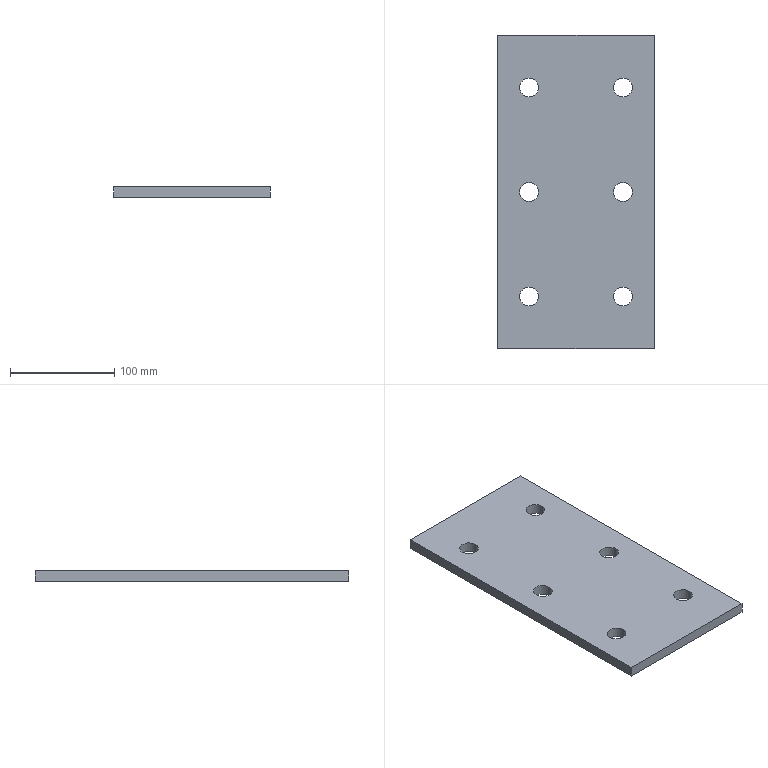Part | SolidWorks | features Extrusion 1 | 1 solid | 18 faces | box 150 x 300 x 10 mm | volume 434732 mm3 | cylinder 12 | plane 6 | commonest cylinder face diameters 18 x12
STEP:
#1=CARTESIAN_POINT('',(36.,100.,10.));
#2=VERTEX_POINT('',#1);
#3=CARTESIAN_POINT('',(54.,100.,10.));
#4=VERTEX_POINT('',#3);
#5=CARTESIAN_POINT('',(45.,100.,10.));
#6=DIRECTION('',(0.,0.,1.));
#7=DIRECTION('',(-1.,0.,0.));
#8=AXIS2_PLACEMENT_3D('',#5,#6,#7);
#9=CIRCLE('',#8,9.);
#10=EDGE_CURVE('',#2,#4,#9,.T.);
#11=ORIENTED_EDGE('',*,*,#10,.T.);
#12=CARTESIAN_POINT('',(54.,100.,0.));
#13=VERTEX_POINT('',#12);
#14=CARTESIAN_POINT('',(54.,100.,10.));
#15=DIRECTION('',(0.,0.,-1.));
#16=VECTOR('',#15,1000.);
#17=LINE('',#14,#16);
#18=EDGE_CURVE('',#4,#13,#17,.T.);
#19=ORIENTED_EDGE('',*,*,#18,.T.);
#20=CARTESIAN_POINT('',(36.,100.,0.));
#21=VERTEX_POINT('',#20);
#22=CARTESIAN_POINT('',(45.,100.,0.));
#23=DIRECTION('',(0.,0.,1.));
#24=DIRECTION('',(-1.,0.,0.));
#25=AXIS2_PLACEMENT_3D('',#22,#23,#24);
#26=CIRCLE('',#25,9.);
#27=EDGE_CURVE('',#21,#13,#26,.T.);
#28=ORIENTED_EDGE('',*,*,#27,.F.);
#29=CARTESIAN_POINT('',(36.,100.,10.));
#30=DIRECTION('',(0.,0.,-1.));
#31=VECTOR('',#30,1000.);
#32=LINE('',#29,#31);
#33=EDGE_CURVE('',#2,#21,#32,.T.);
#34=ORIENTED_EDGE('',*,*,#33,.F.);
#35=EDGE_LOOP('',(#11,#19,#28,#34));
#36=FACE_OUTER_BOUND('',#35,.T.);
#37=CARTESIAN_POINT('',(45.,100.,10.));
#38=DIRECTION('',(0.,0.,-1.));
#39=DIRECTION('',(-1.,0.,0.));
#40=AXIS2_PLACEMENT_3D('',#37,#38,#39);
#41=CYLINDRICAL_SURFACE('',#40,9.);
#42=ADVANCED_FACE('',(#36),#41,.F.);
#43=CARTESIAN_POINT('',(36.,0.,10.));
#44=VERTEX_POINT('',#43);
#45=CARTESIAN_POINT('',(54.,0.,10.));
#46=VERTEX_POINT('',#45);
#47=CARTESIAN_POINT('',(45.,0.,10.));
#48=DIRECTION('',(0.,0.,1.));
#49=DIRECTION('',(-1.,0.,0.));
#50=AXIS2_PLACEMENT_3D('',#47,#48,#49);
#51=CIRCLE('',#50,9.);
#52=EDGE_CURVE('',#44,#46,#51,.T.);
#53=ORIENTED_EDGE('',*,*,#52,.T.);
#54=CARTESIAN_POINT('',(54.,0.,0.));
#55=VERTEX_POINT('',#54);
#56=CARTESIAN_POINT('',(54.,0.,10.));
#57=DIRECTION('',(0.,0.,-1.));
#58=VECTOR('',#57,1000.);
#59=LINE('',#56,#58);
#60=EDGE_CURVE('',#46,#55,#59,.T.);
#61=ORIENTED_EDGE('',*,*,#60,.T.);
#62=CARTESIAN_POINT('',(36.,0.,0.));
#63=VERTEX_POINT('',#62);
#64=CARTESIAN_POINT('',(45.,0.,0.));
#65=DIRECTION('',(0.,0.,1.));
#66=DIRECTION('',(-1.,0.,0.));
#67=AXIS2_PLACEMENT_3D('',#64,#65,#66);
#68=CIRCLE('',#67,9.);
#69=EDGE_CURVE('',#63,#55,#68,.T.);
#70=ORIENTED_EDGE('',*,*,#69,.F.);
#71=CARTESIAN_POINT('',(36.,0.,10.));
#72=DIRECTION('',(0.,0.,-1.));
#73=VECTOR('',#72,1000.);
#74=LINE('',#71,#73);
#75=EDGE_CURVE('',#44,#63,#74,.T.);
#76=ORIENTED_EDGE('',*,*,#75,.F.);
#77=EDGE_LOOP('',(#53,#61,#70,#76));
#78=FACE_OUTER_BOUND('',#77,.T.);
#79=CARTESIAN_POINT('',(45.,0.,10.));
#80=DIRECTION('',(0.,0.,-1.));
#81=DIRECTION('',(-1.,0.,0.));
#82=AXIS2_PLACEMENT_3D('',#79,#80,#81);
#83=CYLINDRICAL_SURFACE('',#82,9.);
#84=ADVANCED_FACE('',(#78),#83,.F.);
#85=CARTESIAN_POINT('',(36.,-100.,10.));
#86=VERTEX_POINT('',#85);
#87=CARTESIAN_POINT('',(54.,-100.,10.));
#88=VERTEX_POINT('',#87);
#89=CARTESIAN_POINT('',(45.,-100.,10.));
#90=DIRECTION('',(0.,0.,1.));
#91=DIRECTION('',(-1.,0.,0.));
#92=AXIS2_PLACEMENT_3D('',#89,#90,#91);
#93=CIRCLE('',#92,9.);
#94=EDGE_CURVE('',#86,#88,#93,.T.);
#95=ORIENTED_EDGE('',*,*,#94,.T.);
#96=CARTESIAN_POINT('',(54.,-100.,0.));
#97=VERTEX_POINT('',#96);
#98=CARTESIAN_POINT('',(54.,-100.,10.));
#99=DIRECTION('',(0.,0.,-1.));
#100=VECTOR('',#99,1000.);
#101=LINE('',#98,#100);
#102=EDGE_CURVE('',#88,#97,#101,.T.);
#103=ORIENTED_EDGE('',*,*,#102,.T.);
#104=CARTESIAN_POINT('',(36.,-100.,0.));
#105=VERTEX_POINT('',#104);
#106=CARTESIAN_POINT('',(45.,-100.,0.));
#107=DIRECTION('',(0.,0.,1.));
#108=DIRECTION('',(-1.,0.,0.));
#109=AXIS2_PLACEMENT_3D('',#106,#107,#108);
#110=CIRCLE('',#109,9.);
#111=EDGE_CURVE('',#105,#97,#110,.T.);
#112=ORIENTED_EDGE('',*,*,#111,.F.);
#113=CARTESIAN_POINT('',(36.,-100.,10.));
#114=DIRECTION('',(0.,0.,-1.));
#115=VECTOR('',#114,1000.);
#116=LINE('',#113,#115);
#117=EDGE_CURVE('',#86,#105,#116,.T.);
#118=ORIENTED_EDGE('',*,*,#117,.F.);
#119=EDGE_LOOP('',(#95,#103,#112,#118));
#120=FACE_OUTER_BOUND('',#119,.T.);
#121=CARTESIAN_POINT('',(45.,-100.,10.));
#122=DIRECTION('',(0.,0.,-1.));
#123=DIRECTION('',(-1.,0.,0.));
#124=AXIS2_PLACEMENT_3D('',#121,#122,#123);
#125=CYLINDRICAL_SURFACE('',#124,9.);
#126=ADVANCED_FACE('',(#120),#125,.F.);
#127=CARTESIAN_POINT('',(-54.,-100.,10.));
#128=VERTEX_POINT('',#127);
#129=CARTESIAN_POINT('',(-36.,-100.,10.));
#130=VERTEX_POINT('',#129);
#131=CARTESIAN_POINT('',(-45.,-100.,10.));
#132=DIRECTION('',(0.,0.,1.));
#133=DIRECTION('',(1.,0.,0.));
#134=AXIS2_PLACEMENT_3D('',#131,#132,#133);
#135=CIRCLE('',#134,9.);
#136=EDGE_CURVE('',#128,#130,#135,.T.);
#137=ORIENTED_EDGE('',*,*,#136,.T.);
#138=CARTESIAN_POINT('',(-36.,-100.,0.));
#139=VERTEX_POINT('',#138);
#140=CARTESIAN_POINT('',(-36.,-100.,10.));
#141=DIRECTION('',(0.,0.,-1.));
#142=VECTOR('',#141,1000.);
#143=LINE('',#140,#142);
#144=EDGE_CURVE('',#130,#139,#143,.T.);
#145=ORIENTED_EDGE('',*,*,#144,.T.);
#146=CARTESIAN_POINT('',(-54.,-100.,0.));
#147=VERTEX_POINT('',#146);
#148=CARTESIAN_POINT('',(-45.,-100.,0.));
#149=DIRECTION('',(0.,0.,1.));
#150=DIRECTION('',(1.,0.,0.));
#151=AXIS2_PLACEMENT_3D('',#148,#149,#150);
#152=CIRCLE('',#151,9.);
#153=EDGE_CURVE('',#147,#139,#152,.T.);
#154=ORIENTED_EDGE('',*,*,#153,.F.);
#155=CARTESIAN_POINT('',(-54.,-100.,10.));
#156=DIRECTION('',(0.,0.,-1.));
#157=VECTOR('',#156,1000.);
#158=LINE('',#155,#157);
#159=EDGE_CURVE('',#128,#147,#158,.T.);
#160=ORIENTED_EDGE('',*,*,#159,.F.);
#161=EDGE_LOOP('',(#137,#145,#154,#160));
#162=FACE_OUTER_BOUND('',#161,.T.);
#163=CARTESIAN_POINT('',(-45.,-100.,10.));
#164=DIRECTION('',(0.,0.,-1.));
#165=DIRECTION('',(-1.,0.,0.));
#166=AXIS2_PLACEMENT_3D('',#163,#164,#165);
#167=CYLINDRICAL_SURFACE('',#166,9.);
#168=ADVANCED_FACE('',(#162),#167,.F.);
#169=CARTESIAN_POINT('',(-54.,0.,10.));
#170=VERTEX_POINT('',#169);
#171=CARTESIAN_POINT('',(-36.,0.,10.));
#172=VERTEX_POINT('',#171);
#173=CARTESIAN_POINT('',(-45.,0.,10.));
#174=DIRECTION('',(0.,0.,1.));
#175=DIRECTION('',(1.,0.,0.));
#176=AXIS2_PLACEMENT_3D('',#173,#174,#175);
#177=CIRCLE('',#176,9.);
#178=EDGE_CURVE('',#170,#172,#177,.T.);
#179=ORIENTED_EDGE('',*,*,#178,.T.);
#180=CARTESIAN_POINT('',(-36.,0.,0.));
#181=VERTEX_POINT('',#180);
#182=CARTESIAN_POINT('',(-36.,0.,10.));
#183=DIRECTION('',(0.,0.,-1.));
#184=VECTOR('',#183,1000.);
#185=LINE('',#182,#184);
#186=EDGE_CURVE('',#172,#181,#185,.T.);
#187=ORIENTED_EDGE('',*,*,#186,.T.);
#188=CARTESIAN_POINT('',(-54.,0.,0.));
#189=VERTEX_POINT('',#188);
#190=CARTESIAN_POINT('',(-45.,0.,0.));
#191=DIRECTION('',(0.,0.,1.));
#192=DIRECTION('',(1.,0.,0.));
#193=AXIS2_PLACEMENT_3D('',#190,#191,#192);
#194=CIRCLE('',#193,9.);
#195=EDGE_CURVE('',#189,#181,#194,.T.);
#196=ORIENTED_EDGE('',*,*,#195,.F.);
#197=CARTESIAN_POINT('',(-54.,0.,10.));
#198=DIRECTION('',(0.,0.,-1.));
#199=VECTOR('',#198,1000.);
#200=LINE('',#197,#199);
#201=EDGE_CURVE('',#170,#189,#200,.T.);
#202=ORIENTED_EDGE('',*,*,#201,.F.);
#203=EDGE_LOOP('',(#179,#187,#196,#202));
#204=FACE_OUTER_BOUND('',#203,.T.);
#205=CARTESIAN_POINT('',(-45.,0.,10.));
#206=DIRECTION('',(0.,0.,-1.));
#207=DIRECTION('',(-1.,0.,0.));
#208=AXIS2_PLACEMENT_3D('',#205,#206,#207);
#209=CYLINDRICAL_SURFACE('',#208,9.);
#210=ADVANCED_FACE('',(#204),#209,.F.);
#211=CARTESIAN_POINT('',(-54.,100.,10.));
#212=VERTEX_POINT('',#211);
#213=CARTESIAN_POINT('',(-36.,100.,10.));
#214=VERTEX_POINT('',#213);
#215=CARTESIAN_POINT('',(-45.,100.,10.));
#216=DIRECTION('',(0.,0.,1.));
#217=DIRECTION('',(1.,0.,0.));
#218=AXIS2_PLACEMENT_3D('',#215,#216,#217);
#219=CIRCLE('',#218,9.);
#220=EDGE_CURVE('',#212,#214,#219,.T.);
#221=ORIENTED_EDGE('',*,*,#220,.T.);
#222=CARTESIAN_POINT('',(-36.,100.,0.));
#223=VERTEX_POINT('',#222);
#224=CARTESIAN_POINT('',(-36.,100.,10.));
#225=DIRECTION('',(0.,0.,-1.));
#226=VECTOR('',#225,1000.);
#227=LINE('',#224,#226);
#228=EDGE_CURVE('',#214,#223,#227,.T.);
#229=ORIENTED_EDGE('',*,*,#228,.T.);
#230=CARTESIAN_POINT('',(-54.,100.,0.));
#231=VERTEX_POINT('',#230);
#232=CARTESIAN_POINT('',(-45.,100.,0.));
#233=DIRECTION('',(0.,0.,1.));
#234=DIRECTION('',(1.,0.,0.));
#235=AXIS2_PLACEMENT_3D('',#232,#233,#234);
#236=CIRCLE('',#235,9.);
#237=EDGE_CURVE('',#231,#223,#236,.T.);
#238=ORIENTED_EDGE('',*,*,#237,.F.);
#239=CARTESIAN_POINT('',(-54.,100.,10.));
#240=DIRECTION('',(0.,0.,-1.));
#241=VECTOR('',#240,1000.);
#242=LINE('',#239,#241);
#243=EDGE_CURVE('',#212,#231,#242,.T.);
#244=ORIENTED_EDGE('',*,*,#243,.F.);
#245=EDGE_LOOP('',(#221,#229,#238,#244));
#246=FACE_OUTER_BOUND('',#245,.T.);
#247=CARTESIAN_POINT('',(-45.,100.,10.));
#248=DIRECTION('',(0.,0.,-1.));
#249=DIRECTION('',(-1.,0.,0.));
#250=AXIS2_PLACEMENT_3D('',#247,#248,#249);
#251=CYLINDRICAL_SURFACE('',#250,9.);
#252=ADVANCED_FACE('',(#246),#251,.F.);
#253=CARTESIAN_POINT('',(-75.,150.,10.));
#254=VERTEX_POINT('',#253);
#255=CARTESIAN_POINT('',(-75.,-150.,10.));
#256=VERTEX_POINT('',#255);
#257=CARTESIAN_POINT('',(-75.,150.,10.));
#258=DIRECTION('',(0.,-1.,0.));
#259=VECTOR('',#258,1000.);
#260=LINE('',#257,#259);
#261=EDGE_CURVE('',#254,#256,#260,.T.);
#262=ORIENTED_EDGE('',*,*,#261,.T.);
#263=CARTESIAN_POINT('',(75.,-150.,10.));
#264=VERTEX_POINT('',#263);
#265=CARTESIAN_POINT('',(75.,-150.,10.));
#266=DIRECTION('',(1.,0.,0.));
#267=VECTOR('',#266,1000.);
#268=LINE('',#265,#267);
#269=EDGE_CURVE('',#256,#264,#268,.T.);
#270=ORIENTED_EDGE('',*,*,#269,.T.);
#271=CARTESIAN_POINT('',(75.,150.,10.));
#272=VERTEX_POINT('',#271);
#273=CARTESIAN_POINT('',(75.,150.,10.));
#274=DIRECTION('',(0.,1.,0.));
#275=VECTOR('',#274,1000.);
#276=LINE('',#273,#275);
#277=EDGE_CURVE('',#264,#272,#276,.T.);
#278=ORIENTED_EDGE('',*,*,#277,.T.);
#279=CARTESIAN_POINT('',(75.,150.,10.));
#280=DIRECTION('',(-1.,0.,0.));
#281=VECTOR('',#280,1000.);
#282=LINE('',#279,#281);
#283=EDGE_CURVE('',#272,#254,#282,.T.);
#284=ORIENTED_EDGE('',*,*,#283,.T.);
#285=EDGE_LOOP('',(#262,#270,#278,#284));
#286=FACE_OUTER_BOUND('',#285,.T.);
#287=ORIENTED_EDGE('',*,*,#220,.F.);
#288=CARTESIAN_POINT('',(-45.,100.,10.));
#289=DIRECTION('',(0.,0.,1.));
#290=DIRECTION('',(1.,0.,0.));
#291=AXIS2_PLACEMENT_3D('',#288,#289,#290);
#292=CIRCLE('',#291,9.);
#293=EDGE_CURVE('',#214,#212,#292,.T.);
#294=ORIENTED_EDGE('',*,*,#293,.F.);
#295=EDGE_LOOP('',(#287,#294));
#296=FACE_BOUND('',#295,.T.);
#297=ORIENTED_EDGE('',*,*,#178,.F.);
#298=CARTESIAN_POINT('',(-45.,0.,10.));
#299=DIRECTION('',(0.,0.,1.));
#300=DIRECTION('',(1.,0.,0.));
#301=AXIS2_PLACEMENT_3D('',#298,#299,#300);
#302=CIRCLE('',#301,9.);
#303=EDGE_CURVE('',#172,#170,#302,.T.);
#304=ORIENTED_EDGE('',*,*,#303,.F.);
#305=EDGE_LOOP('',(#297,#304));
#306=FACE_BOUND('',#305,.T.);
#307=ORIENTED_EDGE('',*,*,#136,.F.);
#308=CARTESIAN_POINT('',(-45.,-100.,10.));
#309=DIRECTION('',(0.,0.,1.));
#310=DIRECTION('',(1.,0.,0.));
#311=AXIS2_PLACEMENT_3D('',#308,#309,#310);
#312=CIRCLE('',#311,9.);
#313=EDGE_CURVE('',#130,#128,#312,.T.);
#314=ORIENTED_EDGE('',*,*,#313,.F.);
#315=EDGE_LOOP('',(#307,#314));
#316=FACE_BOUND('',#315,.T.);
#317=ORIENTED_EDGE('',*,*,#94,.F.);
#318=CARTESIAN_POINT('',(45.,-100.,10.));
#319=DIRECTION('',(0.,0.,1.));
#320=DIRECTION('',(-1.,0.,0.));
#321=AXIS2_PLACEMENT_3D('',#318,#319,#320);
#322=CIRCLE('',#321,9.);
#323=EDGE_CURVE('',#88,#86,#322,.T.);
#324=ORIENTED_EDGE('',*,*,#323,.F.);
#325=EDGE_LOOP('',(#317,#324));
#326=FACE_BOUND('',#325,.T.);
#327=ORIENTED_EDGE('',*,*,#52,.F.);
#328=CARTESIAN_POINT('',(45.,0.,10.));
#329=DIRECTION('',(0.,0.,1.));
#330=DIRECTION('',(-1.,0.,0.));
#331=AXIS2_PLACEMENT_3D('',#328,#329,#330);
#332=CIRCLE('',#331,9.);
#333=EDGE_CURVE('',#46,#44,#332,.T.);
#334=ORIENTED_EDGE('',*,*,#333,.F.);
#335=EDGE_LOOP('',(#327,#334));
#336=FACE_BOUND('',#335,.T.);
#337=ORIENTED_EDGE('',*,*,#10,.F.);
#338=CARTESIAN_POINT('',(45.,100.,10.));
#339=DIRECTION('',(0.,0.,1.));
#340=DIRECTION('',(-1.,0.,0.));
#341=AXIS2_PLACEMENT_3D('',#338,#339,#340);
#342=CIRCLE('',#341,9.);
#343=EDGE_CURVE('',#4,#2,#342,.T.);
#344=ORIENTED_EDGE('',*,*,#343,.F.);
#345=EDGE_LOOP('',(#337,#344));
#346=FACE_BOUND('',#345,.T.);
#347=CARTESIAN_POINT('',(0.,0.,10.));
#348=DIRECTION('',(0.,0.,-1.));
#349=DIRECTION('',(-1.,0.,0.));
#350=AXIS2_PLACEMENT_3D('',#347,#348,#349);
#351=PLANE('',#350);
#352=ADVANCED_FACE('',(#286,#296,#306,#316,#326,#336,#346),#351,.F.);
#353=ORIENTED_EDGE('',*,*,#69,.T.);
#354=CARTESIAN_POINT('',(45.,0.,0.));
#355=DIRECTION('',(0.,0.,1.));
#356=DIRECTION('',(-1.,0.,0.));
#357=AXIS2_PLACEMENT_3D('',#354,#355,#356);
#358=CIRCLE('',#357,9.);
#359=EDGE_CURVE('',#55,#63,#358,.T.);
#360=ORIENTED_EDGE('',*,*,#359,.T.);
#361=EDGE_LOOP('',(#353,#360));
#362=FACE_BOUND('',#361,.T.);
#363=ORIENTED_EDGE('',*,*,#153,.T.);
#364=CARTESIAN_POINT('',(-45.,-100.,0.));
#365=DIRECTION('',(0.,0.,1.));
#366=DIRECTION('',(1.,0.,0.));
#367=AXIS2_PLACEMENT_3D('',#364,#365,#366);
#368=CIRCLE('',#367,9.);
#369=EDGE_CURVE('',#139,#147,#368,.T.);
#370=ORIENTED_EDGE('',*,*,#369,.T.);
#371=EDGE_LOOP('',(#363,#370));
#372=FACE_BOUND('',#371,.T.);
#373=ORIENTED_EDGE('',*,*,#237,.T.);
#374=CARTESIAN_POINT('',(-45.,100.,0.));
#375=DIRECTION('',(0.,0.,1.));
#376=DIRECTION('',(1.,0.,0.));
#377=AXIS2_PLACEMENT_3D('',#374,#375,#376);
#378=CIRCLE('',#377,9.);
#379=EDGE_CURVE('',#223,#231,#378,.T.);
#380=ORIENTED_EDGE('',*,*,#379,.T.);
#381=EDGE_LOOP('',(#373,#380));
#382=FACE_BOUND('',#381,.T.);
#383=CARTESIAN_POINT('',(-75.,150.,0.));
#384=VERTEX_POINT('',#383);
#385=CARTESIAN_POINT('',(-75.,-150.,0.));
#386=VERTEX_POINT('',#385);
#387=CARTESIAN_POINT('',(-75.,150.,0.));
#388=DIRECTION('',(0.,-1.,0.));
#389=VECTOR('',#388,1000.);
#390=LINE('',#387,#389);
#391=EDGE_CURVE('',#384,#386,#390,.T.);
#392=ORIENTED_EDGE('',*,*,#391,.F.);
#393=CARTESIAN_POINT('',(75.,150.,0.));
#394=VERTEX_POINT('',#393);
#395=CARTESIAN_POINT('',(75.,150.,0.));
#396=DIRECTION('',(-1.,0.,0.));
#397=VECTOR('',#396,1000.);
#398=LINE('',#395,#397);
#399=EDGE_CURVE('',#394,#384,#398,.T.);
#400=ORIENTED_EDGE('',*,*,#399,.F.);
#401=CARTESIAN_POINT('',(75.,-150.,0.));
#402=VERTEX_POINT('',#401);
#403=CARTESIAN_POINT('',(75.,150.,0.));
#404=DIRECTION('',(0.,1.,0.));
#405=VECTOR('',#404,1000.);
#406=LINE('',#403,#405);
#407=EDGE_CURVE('',#402,#394,#406,.T.);
#408=ORIENTED_EDGE('',*,*,#407,.F.);
#409=CARTESIAN_POINT('',(75.,-150.,0.));
#410=DIRECTION('',(1.,0.,0.));
#411=VECTOR('',#410,1000.);
#412=LINE('',#409,#411);
#413=EDGE_CURVE('',#386,#402,#412,.T.);
#414=ORIENTED_EDGE('',*,*,#413,.F.);
#415=EDGE_LOOP('',(#392,#400,#408,#414));
#416=FACE_OUTER_BOUND('',#415,.T.);
#417=ORIENTED_EDGE('',*,*,#195,.T.);
#418=CARTESIAN_POINT('',(-45.,0.,0.));
#419=DIRECTION('',(0.,0.,1.));
#420=DIRECTION('',(1.,0.,0.));
#421=AXIS2_PLACEMENT_3D('',#418,#419,#420);
#422=CIRCLE('',#421,9.);
#423=EDGE_CURVE('',#181,#189,#422,.T.);
#424=ORIENTED_EDGE('',*,*,#423,.T.);
#425=EDGE_LOOP('',(#417,#424));
#426=FACE_BOUND('',#425,.T.);
#427=ORIENTED_EDGE('',*,*,#111,.T.);
#428=CARTESIAN_POINT('',(45.,-100.,0.));
#429=DIRECTION('',(0.,0.,1.));
#430=DIRECTION('',(-1.,0.,0.));
#431=AXIS2_PLACEMENT_3D('',#428,#429,#430);
#432=CIRCLE('',#431,9.);
#433=EDGE_CURVE('',#97,#105,#432,.T.);
#434=ORIENTED_EDGE('',*,*,#433,.T.);
#435=EDGE_LOOP('',(#427,#434));
#436=FACE_BOUND('',#435,.T.);
#437=ORIENTED_EDGE('',*,*,#27,.T.);
#438=CARTESIAN_POINT('',(45.,100.,0.));
#439=DIRECTION('',(0.,0.,1.));
#440=DIRECTION('',(-1.,0.,0.));
#441=AXIS2_PLACEMENT_3D('',#438,#439,#440);
#442=CIRCLE('',#441,9.);
#443=EDGE_CURVE('',#13,#21,#442,.T.);
#444=ORIENTED_EDGE('',*,*,#443,.T.);
#445=EDGE_LOOP('',(#437,#444));
#446=FACE_BOUND('',#445,.T.);
#447=CARTESIAN_POINT('',(0.,0.,0.));
#448=DIRECTION('',(0.,0.,-1.));
#449=DIRECTION('',(-1.,0.,0.));
#450=AXIS2_PLACEMENT_3D('',#447,#448,#449);
#451=PLANE('',#450);
#452=ADVANCED_FACE('',(#362,#372,#382,#416,#426,#436,#446),#451,.T.);
#453=ORIENTED_EDGE('',*,*,#391,.T.);
#454=CARTESIAN_POINT('',(-75.,-150.,10.));
#455=DIRECTION('',(0.,0.,-1.));
#456=VECTOR('',#455,1000.);
#457=LINE('',#454,#456);
#458=EDGE_CURVE('',#256,#386,#457,.T.);
#459=ORIENTED_EDGE('',*,*,#458,.F.);
#460=ORIENTED_EDGE('',*,*,#261,.F.);
#461=CARTESIAN_POINT('',(-75.,150.,10.));
#462=DIRECTION('',(0.,0.,-1.));
#463=VECTOR('',#462,1000.);
#464=LINE('',#461,#463);
#465=EDGE_CURVE('',#254,#384,#464,.T.);
#466=ORIENTED_EDGE('',*,*,#465,.T.);
#467=EDGE_LOOP('',(#453,#459,#460,#466));
#468=FACE_OUTER_BOUND('',#467,.T.);
#469=CARTESIAN_POINT('',(-75.,150.,10.));
#470=DIRECTION('',(1.,0.,0.));
#471=DIRECTION('',(0.,1.,0.));
#472=AXIS2_PLACEMENT_3D('',#469,#470,#471);
#473=PLANE('',#472);
#474=ADVANCED_FACE('',(#468),#473,.F.);
#475=ORIENTED_EDGE('',*,*,#413,.T.);
#476=CARTESIAN_POINT('',(75.,-150.,10.));
#477=DIRECTION('',(0.,0.,-1.));
#478=VECTOR('',#477,1000.);
#479=LINE('',#476,#478);
#480=EDGE_CURVE('',#264,#402,#479,.T.);
#481=ORIENTED_EDGE('',*,*,#480,.F.);
#482=ORIENTED_EDGE('',*,*,#269,.F.);
#483=ORIENTED_EDGE('',*,*,#458,.T.);
#484=EDGE_LOOP('',(#475,#481,#482,#483));
#485=FACE_OUTER_BOUND('',#484,.T.);
#486=CARTESIAN_POINT('',(75.,-150.,10.));
#487=DIRECTION('',(0.,1.,0.));
#488=DIRECTION('',(-1.,0.,0.));
#489=AXIS2_PLACEMENT_3D('',#486,#487,#488);
#490=PLANE('',#489);
#491=ADVANCED_FACE('',(#485),#490,.F.);
#492=ORIENTED_EDGE('',*,*,#407,.T.);
#493=CARTESIAN_POINT('',(75.,150.,10.));
#494=DIRECTION('',(0.,0.,-1.));
#495=VECTOR('',#494,1000.);
#496=LINE('',#493,#495);
#497=EDGE_CURVE('',#272,#394,#496,.T.);
#498=ORIENTED_EDGE('',*,*,#497,.F.);
#499=ORIENTED_EDGE('',*,*,#277,.F.);
#500=ORIENTED_EDGE('',*,*,#480,.T.);
#501=EDGE_LOOP('',(#492,#498,#499,#500));
#502=FACE_OUTER_BOUND('',#501,.T.);
#503=CARTESIAN_POINT('',(75.,150.,10.));
#504=DIRECTION('',(-1.,0.,0.));
#505=DIRECTION('',(0.,-1.,0.));
#506=AXIS2_PLACEMENT_3D('',#503,#504,#505);
#507=PLANE('',#506);
#508=ADVANCED_FACE('',(#502),#507,.F.);
#509=ORIENTED_EDGE('',*,*,#399,.T.);
#510=ORIENTED_EDGE('',*,*,#465,.F.);
#511=ORIENTED_EDGE('',*,*,#283,.F.);
#512=ORIENTED_EDGE('',*,*,#497,.T.);
#513=EDGE_LOOP('',(#509,#510,#511,#512));
#514=FACE_OUTER_BOUND('',#513,.T.);
#515=CARTESIAN_POINT('',(75.,150.,10.));
#516=DIRECTION('',(0.,-1.,0.));
#517=DIRECTION('',(1.,0.,0.));
#518=AXIS2_PLACEMENT_3D('',#515,#516,#517);
#519=PLANE('',#518);
#520=ADVANCED_FACE('',(#514),#519,.F.);
#521=ORIENTED_EDGE('',*,*,#228,.F.);
#522=ORIENTED_EDGE('',*,*,#293,.T.);
#523=ORIENTED_EDGE('',*,*,#243,.T.);
#524=ORIENTED_EDGE('',*,*,#379,.F.);
#525=EDGE_LOOP('',(#521,#522,#523,#524));
#526=FACE_OUTER_BOUND('',#525,.T.);
#527=CARTESIAN_POINT('',(-45.,100.,10.));
#528=DIRECTION('',(0.,0.,-1.));
#529=DIRECTION('',(-1.,0.,0.));
#530=AXIS2_PLACEMENT_3D('',#527,#528,#529);
#531=CYLINDRICAL_SURFACE('',#530,9.);
#532=ADVANCED_FACE('',(#526),#531,.F.);
#533=ORIENTED_EDGE('',*,*,#186,.F.);
#534=ORIENTED_EDGE('',*,*,#303,.T.);
#535=ORIENTED_EDGE('',*,*,#201,.T.);
#536=ORIENTED_EDGE('',*,*,#423,.F.);
#537=EDGE_LOOP('',(#533,#534,#535,#536));
#538=FACE_OUTER_BOUND('',#537,.T.);
#539=CARTESIAN_POINT('',(-45.,0.,10.));
#540=DIRECTION('',(0.,0.,-1.));
#541=DIRECTION('',(-1.,0.,0.));
#542=AXIS2_PLACEMENT_3D('',#539,#540,#541);
#543=CYLINDRICAL_SURFACE('',#542,9.);
#544=ADVANCED_FACE('',(#538),#543,.F.);
#545=ORIENTED_EDGE('',*,*,#144,.F.);
#546=ORIENTED_EDGE('',*,*,#313,.T.);
#547=ORIENTED_EDGE('',*,*,#159,.T.);
#548=ORIENTED_EDGE('',*,*,#369,.F.);
#549=EDGE_LOOP('',(#545,#546,#547,#548));
#550=FACE_OUTER_BOUND('',#549,.T.);
#551=CARTESIAN_POINT('',(-45.,-100.,10.));
#552=DIRECTION('',(0.,0.,-1.));
#553=DIRECTION('',(-1.,0.,0.));
#554=AXIS2_PLACEMENT_3D('',#551,#552,#553);
#555=CYLINDRICAL_SURFACE('',#554,9.);
#556=ADVANCED_FACE('',(#550),#555,.F.);
#557=ORIENTED_EDGE('',*,*,#102,.F.);
#558=ORIENTED_EDGE('',*,*,#323,.T.);
#559=ORIENTED_EDGE('',*,*,#117,.T.);
#560=ORIENTED_EDGE('',*,*,#433,.F.);
#561=EDGE_LOOP('',(#557,#558,#559,#560));
#562=FACE_OUTER_BOUND('',#561,.T.);
#563=CARTESIAN_POINT('',(45.,-100.,10.));
#564=DIRECTION('',(0.,0.,-1.));
#565=DIRECTION('',(-1.,0.,0.));
#566=AXIS2_PLACEMENT_3D('',#563,#564,#565);
#567=CYLINDRICAL_SURFACE('',#566,9.);
#568=ADVANCED_FACE('',(#562),#567,.F.);
#569=ORIENTED_EDGE('',*,*,#60,.F.);
#570=ORIENTED_EDGE('',*,*,#333,.T.);
#571=ORIENTED_EDGE('',*,*,#75,.T.);
#572=ORIENTED_EDGE('',*,*,#359,.F.);
#573=EDGE_LOOP('',(#569,#570,#571,#572));
#574=FACE_OUTER_BOUND('',#573,.T.);
#575=CARTESIAN_POINT('',(45.,0.,10.));
#576=DIRECTION('',(0.,0.,-1.));
#577=DIRECTION('',(-1.,0.,0.));
#578=AXIS2_PLACEMENT_3D('',#575,#576,#577);
#579=CYLINDRICAL_SURFACE('',#578,9.);
#580=ADVANCED_FACE('',(#574),#579,.F.);
#581=ORIENTED_EDGE('',*,*,#18,.F.);
#582=ORIENTED_EDGE('',*,*,#343,.T.);
#583=ORIENTED_EDGE('',*,*,#33,.T.);
#584=ORIENTED_EDGE('',*,*,#443,.F.);
#585=EDGE_LOOP('',(#581,#582,#583,#584));
#586=FACE_OUTER_BOUND('',#585,.T.);
#587=CARTESIAN_POINT('',(45.,100.,10.));
#588=DIRECTION('',(0.,0.,-1.));
#589=DIRECTION('',(-1.,0.,0.));
#590=AXIS2_PLACEMENT_3D('',#587,#588,#589);
#591=CYLINDRICAL_SURFACE('',#590,9.);
#592=ADVANCED_FACE('',(#586),#591,.F.);
#593=CLOSED_SHELL('',(#42,#84,#126,#168,#210,#252,#352,#452,#474,#491,#508,#520,#532,#544,#556,#568,#580,#592));
#594=MANIFOLD_SOLID_BREP('',#593);
#595=CARTESIAN_POINT('',(0.,0.,0.));
#596=DIRECTION('',(0.,0.,1.));
#597=DIRECTION('',(1.,0.,0.));
#598=AXIS2_PLACEMENT_3D('',#595,#596,#597);
#599=(LENGTH_UNIT()NAMED_UNIT(*)SI_UNIT(.MILLI.,.METRE.));
#600=UNCERTAINTY_MEASURE_WITH_UNIT(LENGTH_MEASURE(0.00001),#599,'','');
#601=(NAMED_UNIT(*)PLANE_ANGLE_UNIT()SI_UNIT($,.RADIAN.));
#602=(NAMED_UNIT(*)SI_UNIT($,.STERADIAN.)SOLID_ANGLE_UNIT());
#603=(GEOMETRIC_REPRESENTATION_CONTEXT(3)GLOBAL_UNCERTAINTY_ASSIGNED_CONTEXT((#600))GLOBAL_UNIT_ASSIGNED_CONTEXT((#599,#601,#602))REPRESENTATION_CONTEXT('',''));
#604=ADVANCED_BREP_SHAPE_REPRESENTATION('',(#594,#598),#603);